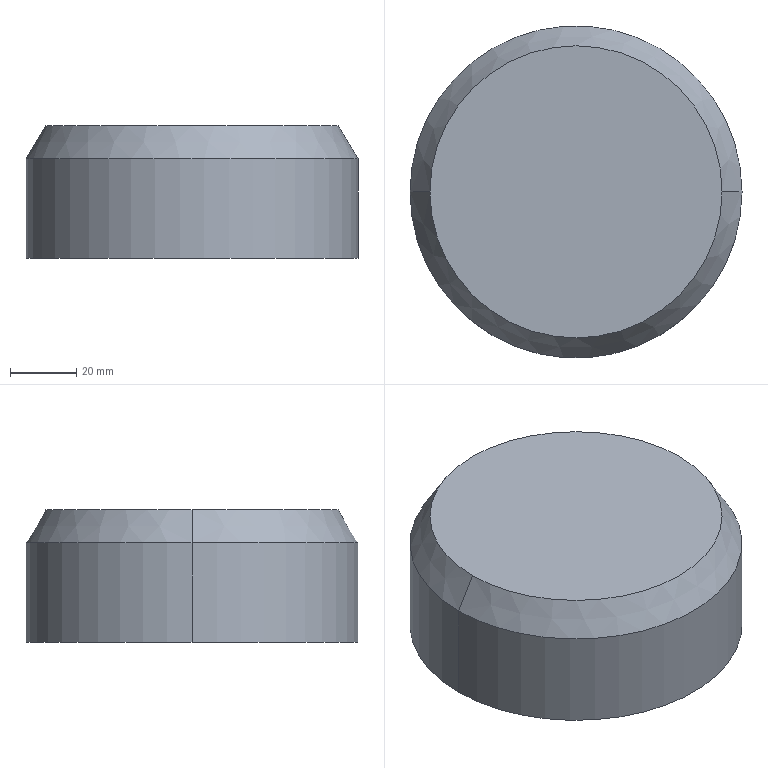Part | SolidWorks | features Chamfer 1, Extrusion 1, HoleWzd 1 | 1 solid | 10 faces | box 100 x 100 x 40 mm | volume 304768 mm3 | cylinder 4 | cone 4 | plane 2 | commonest cylinder face diameters 5 x2 100 x2
STEP:
#1=CARTESIAN_POINT('',(2.5,0.,17.));
#2=VERTEX_POINT('',#1);
#3=CARTESIAN_POINT('',(-2.5,0.,17.));
#4=VERTEX_POINT('',#3);
#5=CARTESIAN_POINT('',(0.,0.,17.));
#6=DIRECTION('',(0.,0.,-1.));
#7=DIRECTION('',(-1.,0.,0.));
#8=AXIS2_PLACEMENT_3D('',#5,#6,#7);
#9=CIRCLE('',#8,2.5);
#10=EDGE_CURVE('',#2,#4,#9,.T.);
#11=ORIENTED_EDGE('',*,*,#10,.F.);
#12=CARTESIAN_POINT('',(2.5,0.,0.));
#13=VERTEX_POINT('',#12);
#14=CARTESIAN_POINT('',(2.5,0.,0.));
#15=DIRECTION('',(0.,0.,-1.));
#16=VECTOR('',#15,1000.);
#17=LINE('',#14,#16);
#18=EDGE_CURVE('',#2,#13,#17,.T.);
#19=ORIENTED_EDGE('',*,*,#18,.T.);
#20=CARTESIAN_POINT('',(-2.5,0.,0.));
#21=VERTEX_POINT('',#20);
#22=CARTESIAN_POINT('',(0.,0.,0.));
#23=DIRECTION('',(0.,0.,-1.));
#24=DIRECTION('',(-1.,0.,0.));
#25=AXIS2_PLACEMENT_3D('',#22,#23,#24);
#26=CIRCLE('',#25,2.5);
#27=EDGE_CURVE('',#13,#21,#26,.T.);
#28=ORIENTED_EDGE('',*,*,#27,.T.);
#29=CARTESIAN_POINT('',(-2.5,0.,0.));
#30=DIRECTION('',(0.,0.,-1.));
#31=VECTOR('',#30,1000.);
#32=LINE('',#29,#31);
#33=EDGE_CURVE('',#4,#21,#32,.T.);
#34=ORIENTED_EDGE('',*,*,#33,.F.);
#35=EDGE_LOOP('',(#11,#19,#28,#34));
#36=FACE_OUTER_BOUND('',#35,.T.);
#37=CARTESIAN_POINT('',(0.,0.,0.));
#38=DIRECTION('',(0.,0.,-1.));
#39=DIRECTION('',(-1.,0.,0.));
#40=AXIS2_PLACEMENT_3D('',#37,#38,#39);
#41=CYLINDRICAL_SURFACE('',#40,2.5);
#42=ADVANCED_FACE('',(#36),#41,.F.);
#43=CARTESIAN_POINT('',(0.,0.,18.502));
#44=VERTEX_POINT('',#43);
#45=CARTESIAN_POINT('',(-2.5,0.,17.));
#46=DIRECTION('',(-0.8572,0.,-0.515));
#47=VECTOR('',#46,1000.);
#48=LINE('',#45,#47);
#49=EDGE_CURVE('',#44,#4,#48,.T.);
#50=ORIENTED_EDGE('',*,*,#49,.F.);
#51=CARTESIAN_POINT('',(2.5,0.,17.));
#52=DIRECTION('',(0.8572,0.,-0.515));
#53=VECTOR('',#52,1000.);
#54=LINE('',#51,#53);
#55=EDGE_CURVE('',#44,#2,#54,.T.);
#56=ORIENTED_EDGE('',*,*,#55,.T.);
#57=ORIENTED_EDGE('',*,*,#10,.T.);
#58=EDGE_LOOP('',(#50,#56,#57));
#59=FACE_OUTER_BOUND('',#58,.T.);
#60=CARTESIAN_POINT('',(0.,0.,17.));
#61=DIRECTION('',(0.,0.,-1.));
#62=DIRECTION('',(-1.,0.,0.));
#63=AXIS2_PLACEMENT_3D('',#60,#61,#62);
#64=CONICAL_SURFACE('',#63,2.5,1.03);
#65=ADVANCED_FACE('',(#59),#64,.F.);
#66=CARTESIAN_POINT('',(44.,0.,40.));
#67=VERTEX_POINT('',#66);
#68=CARTESIAN_POINT('',(-44.,0.,40.));
#69=VERTEX_POINT('',#68);
#70=CARTESIAN_POINT('',(0.,0.,40.));
#71=DIRECTION('',(0.,0.,1.));
#72=DIRECTION('',(1.,0.,0.));
#73=AXIS2_PLACEMENT_3D('',#70,#71,#72);
#74=CIRCLE('',#73,44.);
#75=EDGE_CURVE('',#67,#69,#74,.T.);
#76=ORIENTED_EDGE('',*,*,#75,.F.);
#77=CARTESIAN_POINT('',(50.,0.,30.));
#78=VERTEX_POINT('',#77);
#79=CARTESIAN_POINT('',(44.,0.,40.));
#80=DIRECTION('',(0.5145,0.,-0.8575));
#81=VECTOR('',#80,1000.);
#82=LINE('',#79,#81);
#83=EDGE_CURVE('',#67,#78,#82,.T.);
#84=ORIENTED_EDGE('',*,*,#83,.T.);
#85=CARTESIAN_POINT('',(-50.,0.,30.));
#86=VERTEX_POINT('',#85);
#87=CARTESIAN_POINT('',(0.,0.,30.));
#88=DIRECTION('',(0.,0.,-1.));
#89=DIRECTION('',(1.,0.,0.));
#90=AXIS2_PLACEMENT_3D('',#87,#88,#89);
#91=CIRCLE('',#90,50.);
#92=EDGE_CURVE('',#86,#78,#91,.T.);
#93=ORIENTED_EDGE('',*,*,#92,.F.);
#94=CARTESIAN_POINT('',(-44.,0.,40.));
#95=DIRECTION('',(-0.5145,0.,-0.8575));
#96=VECTOR('',#95,1000.);
#97=LINE('',#94,#96);
#98=EDGE_CURVE('',#69,#86,#97,.T.);
#99=ORIENTED_EDGE('',*,*,#98,.F.);
#100=EDGE_LOOP('',(#76,#84,#93,#99));
#101=FACE_OUTER_BOUND('',#100,.T.);
#102=CARTESIAN_POINT('',(0.,0.,40.));
#103=DIRECTION('',(0.,0.,-1.));
#104=DIRECTION('',(-1.,0.,0.));
#105=AXIS2_PLACEMENT_3D('',#102,#103,#104);
#106=CONICAL_SURFACE('',#105,44.,0.5404);
#107=ADVANCED_FACE('',(#101),#106,.T.);
#108=ORIENTED_EDGE('',*,*,#92,.T.);
#109=CARTESIAN_POINT('',(50.,0.,0.));
#110=VERTEX_POINT('',#109);
#111=CARTESIAN_POINT('',(50.,0.,40.));
#112=DIRECTION('',(0.,0.,-1.));
#113=VECTOR('',#112,1000.);
#114=LINE('',#111,#113);
#115=EDGE_CURVE('',#78,#110,#114,.T.);
#116=ORIENTED_EDGE('',*,*,#115,.T.);
#117=CARTESIAN_POINT('',(-50.,0.,0.));
#118=VERTEX_POINT('',#117);
#119=CARTESIAN_POINT('',(0.,0.,0.));
#120=DIRECTION('',(0.,0.,1.));
#121=DIRECTION('',(1.,0.,0.));
#122=AXIS2_PLACEMENT_3D('',#119,#120,#121);
#123=CIRCLE('',#122,50.);
#124=EDGE_CURVE('',#110,#118,#123,.T.);
#125=ORIENTED_EDGE('',*,*,#124,.T.);
#126=CARTESIAN_POINT('',(-50.,0.,40.));
#127=DIRECTION('',(0.,0.,-1.));
#128=VECTOR('',#127,1000.);
#129=LINE('',#126,#128);
#130=EDGE_CURVE('',#86,#118,#129,.T.);
#131=ORIENTED_EDGE('',*,*,#130,.F.);
#132=EDGE_LOOP('',(#108,#116,#125,#131));
#133=FACE_OUTER_BOUND('',#132,.T.);
#134=CARTESIAN_POINT('',(0.,0.,40.));
#135=DIRECTION('',(0.,0.,-1.));
#136=DIRECTION('',(-1.,0.,0.));
#137=AXIS2_PLACEMENT_3D('',#134,#135,#136);
#138=CYLINDRICAL_SURFACE('',#137,50.);
#139=ADVANCED_FACE('',(#133),#138,.T.);
#140=ORIENTED_EDGE('',*,*,#115,.F.);
#141=CARTESIAN_POINT('',(0.,0.,30.));
#142=DIRECTION('',(0.,0.,-1.));
#143=DIRECTION('',(1.,0.,0.));
#144=AXIS2_PLACEMENT_3D('',#141,#142,#143);
#145=CIRCLE('',#144,50.);
#146=EDGE_CURVE('',#78,#86,#145,.T.);
#147=ORIENTED_EDGE('',*,*,#146,.T.);
#148=ORIENTED_EDGE('',*,*,#130,.T.);
#149=CARTESIAN_POINT('',(0.,0.,0.));
#150=DIRECTION('',(0.,0.,1.));
#151=DIRECTION('',(1.,0.,0.));
#152=AXIS2_PLACEMENT_3D('',#149,#150,#151);
#153=CIRCLE('',#152,50.);
#154=EDGE_CURVE('',#118,#110,#153,.T.);
#155=ORIENTED_EDGE('',*,*,#154,.T.);
#156=EDGE_LOOP('',(#140,#147,#148,#155));
#157=FACE_OUTER_BOUND('',#156,.T.);
#158=CARTESIAN_POINT('',(0.,0.,40.));
#159=DIRECTION('',(0.,0.,-1.));
#160=DIRECTION('',(-1.,0.,0.));
#161=AXIS2_PLACEMENT_3D('',#158,#159,#160);
#162=CYLINDRICAL_SURFACE('',#161,50.);
#163=ADVANCED_FACE('',(#157),#162,.T.);
#164=CARTESIAN_POINT('',(0.,0.,40.));
#165=DIRECTION('',(0.,0.,1.));
#166=DIRECTION('',(1.,0.,0.));
#167=AXIS2_PLACEMENT_3D('',#164,#165,#166);
#168=CIRCLE('',#167,44.);
#169=EDGE_CURVE('',#69,#67,#168,.T.);
#170=ORIENTED_EDGE('',*,*,#169,.T.);
#171=ORIENTED_EDGE('',*,*,#75,.T.);
#172=EDGE_LOOP('',(#170,#171));
#173=FACE_OUTER_BOUND('',#172,.T.);
#174=CARTESIAN_POINT('',(0.,0.,40.));
#175=DIRECTION('',(0.,0.,1.));
#176=DIRECTION('',(1.,0.,0.));
#177=AXIS2_PLACEMENT_3D('',#174,#175,#176);
#178=PLANE('',#177);
#179=ADVANCED_FACE('',(#173),#178,.T.);
#180=CARTESIAN_POINT('',(0.,0.,0.));
#181=DIRECTION('',(0.,0.,-1.));
#182=DIRECTION('',(-1.,0.,0.));
#183=AXIS2_PLACEMENT_3D('',#180,#181,#182);
#184=CIRCLE('',#183,2.5);
#185=EDGE_CURVE('',#21,#13,#184,.T.);
#186=ORIENTED_EDGE('',*,*,#185,.F.);
#187=ORIENTED_EDGE('',*,*,#27,.F.);
#188=EDGE_LOOP('',(#186,#187));
#189=FACE_BOUND('',#188,.T.);
#190=ORIENTED_EDGE('',*,*,#154,.F.);
#191=ORIENTED_EDGE('',*,*,#124,.F.);
#192=EDGE_LOOP('',(#190,#191));
#193=FACE_OUTER_BOUND('',#192,.T.);
#194=CARTESIAN_POINT('',(0.,0.,0.));
#195=DIRECTION('',(0.,0.,1.));
#196=DIRECTION('',(1.,0.,0.));
#197=AXIS2_PLACEMENT_3D('',#194,#195,#196);
#198=PLANE('',#197);
#199=ADVANCED_FACE('',(#189,#193),#198,.F.);
#200=ORIENTED_EDGE('',*,*,#83,.F.);
#201=ORIENTED_EDGE('',*,*,#169,.F.);
#202=ORIENTED_EDGE('',*,*,#98,.T.);
#203=ORIENTED_EDGE('',*,*,#146,.F.);
#204=EDGE_LOOP('',(#200,#201,#202,#203));
#205=FACE_OUTER_BOUND('',#204,.T.);
#206=CARTESIAN_POINT('',(0.,0.,40.));
#207=DIRECTION('',(0.,0.,-1.));
#208=DIRECTION('',(-1.,0.,0.));
#209=AXIS2_PLACEMENT_3D('',#206,#207,#208);
#210=CONICAL_SURFACE('',#209,44.,0.5404);
#211=ADVANCED_FACE('',(#205),#210,.T.);
#212=ORIENTED_EDGE('',*,*,#55,.F.);
#213=ORIENTED_EDGE('',*,*,#49,.T.);
#214=CARTESIAN_POINT('',(0.,0.,17.));
#215=DIRECTION('',(0.,0.,-1.));
#216=DIRECTION('',(-1.,0.,0.));
#217=AXIS2_PLACEMENT_3D('',#214,#215,#216);
#218=CIRCLE('',#217,2.5);
#219=EDGE_CURVE('',#4,#2,#218,.T.);
#220=ORIENTED_EDGE('',*,*,#219,.T.);
#221=EDGE_LOOP('',(#212,#213,#220));
#222=FACE_OUTER_BOUND('',#221,.T.);
#223=CARTESIAN_POINT('',(0.,0.,17.));
#224=DIRECTION('',(0.,0.,-1.));
#225=DIRECTION('',(-1.,0.,0.));
#226=AXIS2_PLACEMENT_3D('',#223,#224,#225);
#227=CONICAL_SURFACE('',#226,2.5,1.03);
#228=ADVANCED_FACE('',(#222),#227,.F.);
#229=ORIENTED_EDGE('',*,*,#18,.F.);
#230=ORIENTED_EDGE('',*,*,#219,.F.);
#231=ORIENTED_EDGE('',*,*,#33,.T.);
#232=ORIENTED_EDGE('',*,*,#185,.T.);
#233=EDGE_LOOP('',(#229,#230,#231,#232));
#234=FACE_OUTER_BOUND('',#233,.T.);
#235=CARTESIAN_POINT('',(0.,0.,0.));
#236=DIRECTION('',(0.,0.,-1.));
#237=DIRECTION('',(-1.,0.,0.));
#238=AXIS2_PLACEMENT_3D('',#235,#236,#237);
#239=CYLINDRICAL_SURFACE('',#238,2.5);
#240=ADVANCED_FACE('',(#234),#239,.F.);
#241=CLOSED_SHELL('',(#42,#65,#107,#139,#163,#179,#199,#211,#228,#240));
#242=MANIFOLD_SOLID_BREP('',#241);
#243=CARTESIAN_POINT('',(0.,0.,0.));
#244=DIRECTION('',(0.,0.,1.));
#245=DIRECTION('',(1.,0.,0.));
#246=AXIS2_PLACEMENT_3D('',#243,#244,#245);
#247=(LENGTH_UNIT()NAMED_UNIT(*)SI_UNIT(.MILLI.,.METRE.));
#248=UNCERTAINTY_MEASURE_WITH_UNIT(LENGTH_MEASURE(0.00001),#247,'','');
#249=(NAMED_UNIT(*)PLANE_ANGLE_UNIT()SI_UNIT($,.RADIAN.));
#250=(NAMED_UNIT(*)SI_UNIT($,.STERADIAN.)SOLID_ANGLE_UNIT());
#251=(GEOMETRIC_REPRESENTATION_CONTEXT(3)GLOBAL_UNCERTAINTY_ASSIGNED_CONTEXT((#248))GLOBAL_UNIT_ASSIGNED_CONTEXT((#247,#249,#250))REPRESENTATION_CONTEXT('',''));
#252=ADVANCED_BREP_SHAPE_REPRESENTATION('',(#242,#246),#251);